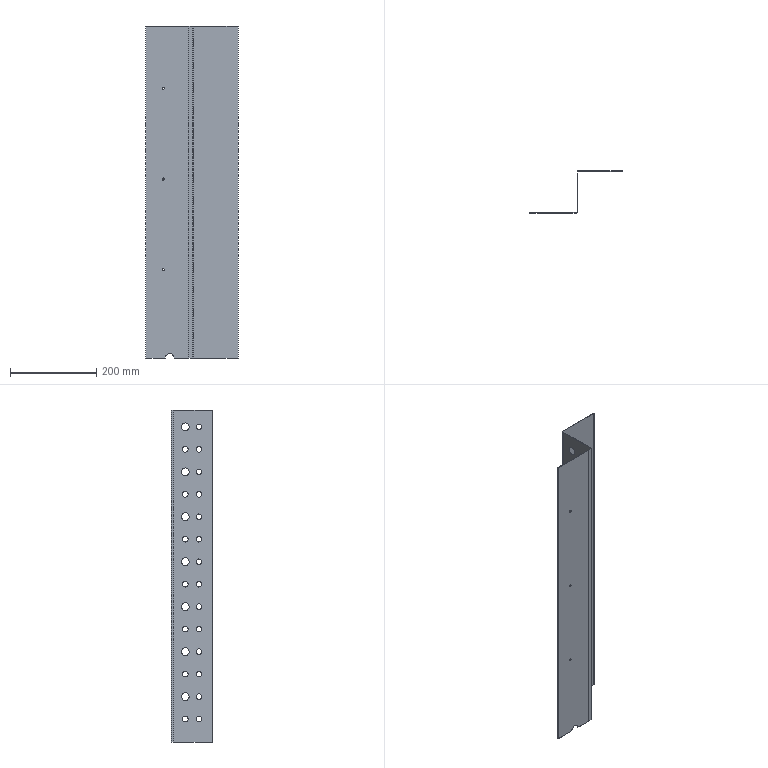Part | STEP file | 64524330 | 1 solid | 94 faces | box 213.75 x 96 x 768 mm | volume 116112 mm3 | cylinder 67 | plane 27 | commonest cylinder face diameters 13 x42 18 x14 5 x6 1 x2 2 x2 20 x1